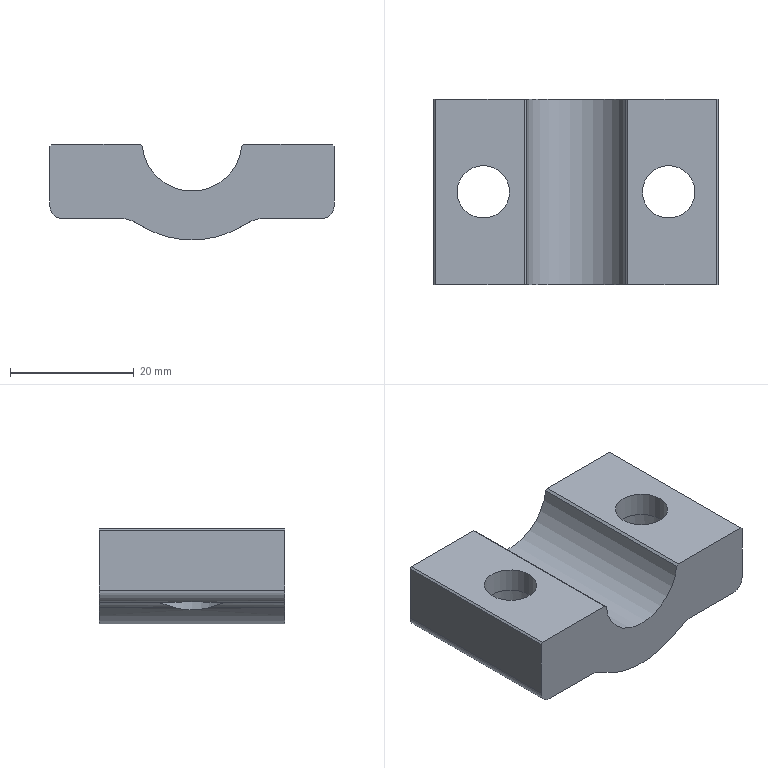NC program | NX | posted with a generic post | part box 46 x 30 x 15.5 mm
Lines 1685 to 1865 of 1865:
(PLANAR_MILL , TOOL : D10精光)
N3362 T03 M6
N3364 G54
N3366 G17 G0 G90 X2.102 Y11.765 B0. C0. S1061 M3
N3368 G43 Z30. H3
N3370 Z-13.5
N3372 G94 G1 Z-15.5 F250.
N3374 G41 X2.208 Y11.595 D3
N3376 G3 X5.033 Y11.456 R2.
N3378 G2 X8.39 Y12.75 R5.
N3380 G1 X22.7
N3382 G2 X26.236 Y11.286 R5.
N3384 G1 X26.536 Y10.986
N3386 G2 X28. Y7.45 R5.
N3388 G1 Y-2.25
N3390 G2 X21. Y-9.25 R7.
N3392 G1 X11.608
N3394 G2 X-11.608 Y-9.25 R21.
N3396 G1 X-21.
N3398 G2 X-28. Y-2.25 R7.
N3400 G1 Y7.45
N3402 G2 X-26.536 Y10.986 R5.
N3404 G1 X-26.236 Y11.286
N3406 G2 X-22.7 Y12.75 R5.
N3408 G1 X-8.39
N3410 G2 X-5.033 Y11.456 R5.
N3412 G1 X-4.704 Y11.157
N3414 G2 X-3.085 Y7.944 R5.
N3416 G3 X3.085 Y7.944 R3.1
N3418 G2 X4.704 Y11.157 R5.
N3420 G1 X5.033 Y11.456
N3422 G3 X5.173 Y14.281 R2.
N3424 G40
N3426 G1 X5.015 Y14.403
N3428 X2.102 Y11.765
N3430 G41 X2.208 Y11.595
N3432 G3 X5.033 Y11.456 R2.
N3434 G2 X8.39 Y12.75 R5.
N3436 G1 X22.7
N3438 G2 X26.236 Y11.286 R5.
N3440 G1 X26.536 Y10.986
N3442 G2 X28. Y7.45 R5.
N3444 G1 Y-2.25
N3446 G2 X21. Y-9.25 R7.
N3448 G1 X11.608
N3450 G2 X-11.608 Y-9.25 R21.
N3452 G1 X-21.
N3454 G2 X-28. Y-2.25 R7.
N3456 G1 Y7.45
N3458 G2 X-26.536 Y10.986 R5.
N3460 G1 X-26.236 Y11.286
N3462 G2 X-22.7 Y12.75 R5.
N3464 G1 X-8.39
N3466 G2 X-5.033 Y11.456 R5.
N3468 G1 X-4.704 Y11.157
N3470 G2 X-3.085 Y7.944 R5.
N3472 G3 X3.085 Y7.944 R3.1
N3474 G2 X4.704 Y11.157 R5.
N3476 G1 X5.033 Y11.456
N3478 G3 X5.173 Y14.281 R2.
N3480 G40
N3482 G1 X5.015 Y14.403
N3484 Z-13.5
N3486 G0 Z30.
N3488 X2.102 Y11.765
N3490 Z-29.
N3492 G1 Z-31.
N3494 G41 X2.208 Y11.595
N3496 G3 X5.033 Y11.456 R2.
N3498 G2 X8.39 Y12.75 R5.
N3500 G1 X22.7
N3502 G2 X26.236 Y11.286 R5.
N3504 G1 X26.536 Y10.986
N3506 G2 X28. Y7.45 R5.
N3508 G1 Y-2.25
N3510 G2 X21. Y-9.25 R7.
N3512 G1 X11.608
N3514 G2 X-11.608 Y-9.25 R21.
N3516 G1 X-21.
N3518 G2 X-28. Y-2.25 R7.
N3520 G1 Y7.45
N3522 G2 X-26.536 Y10.986 R5.
N3524 G1 X-26.236 Y11.286
N3526 G2 X-22.7 Y12.75 R5.
N3528 G1 X-8.39
N3530 G2 X-5.033 Y11.456 R5.
N3532 G1 X-4.704 Y11.157
N3534 G2 X-3.085 Y7.944 R5.
N3536 G3 X3.085 Y7.944 R3.1
N3538 G2 X4.704 Y11.157 R5.
N3540 G1 X5.033 Y11.456
N3542 G3 X5.173 Y14.281 R2.
N3544 G40
N3546 G1 X5.015 Y14.403
N3548 X2.102 Y11.765
N3550 G41 X2.208 Y11.595
N3552 G3 X5.033 Y11.456 R2.
N3554 G2 X8.39 Y12.75 R5.
N3556 G1 X22.7
N3558 G2 X26.236 Y11.286 R5.
N3560 G1 X26.536 Y10.986
N3562 G2 X28. Y7.45 R5.
N3564 G1 Y-2.25
N3566 G2 X21. Y-9.25 R7.
N3568 G1 X11.608
N3570 G2 X-11.608 Y-9.25 R21.
N3572 G1 X-21.
N3574 G2 X-28. Y-2.25 R7.
N3576 G1 Y7.45
N3578 G2 X-26.536 Y10.986 R5.
N3580 G1 X-26.236 Y11.286
N3582 G2 X-22.7 Y12.75 R5.
N3584 G1 X-8.39
N3586 G2 X-5.033 Y11.456 R5.
N3588 G1 X-4.704 Y11.157
N3590 G2 X-3.085 Y7.944 R5.
N3592 G3 X3.085 Y7.944 R3.1
N3594 G2 X4.704 Y11.157 R5.
N3596 G1 X5.033 Y11.456
N3598 G3 X5.173 Y14.281 R2.
N3600 G40
N3602 G1 X5.015 Y14.403
N3604 Z-29.
N3606 G0 Z30.
N3608 M5
(PLANAR_MILL_COPY , TOOL : D10点钻)
N3610 T04 M6
N3612 G54
N3614 G17 G0 G90 X4.222 Y9.372 B0. C0. S3000 M3
N3616 G43 Z30. H4
N3618 Z0.
N3620 G94 G1 Z-2. F800.
N3622 G3 X7.047 Y9.232 R2.
N3624 G2 X8.39 Y9.75 R2.
N3626 G1 X22.7
N3628 G2 X24.114 Y9.164 R2.
N3630 G1 X24.414 Y8.864
N3632 G2 X25. Y7.45 R2.
N3634 G1 Y-2.25
N3636 G2 X21. Y-6.25 R4.
N3638 G1 X11.608
N3640 G3 X9.95 Y-6.75 R3.
N3642 G2 X-9.95 Y-6.75 R18.
N3644 G3 X-11.608 Y-6.25 R3.
N3646 G1 X-21.
N3648 G2 X-25. Y-2.25 R4.
N3650 G1 Y7.45
N3652 G2 X-24.414 Y8.864 R2.
N3654 G1 X-24.114 Y9.164
N3656 G2 X-22.7 Y9.75 R2.
N3658 G1 X-8.39
N3660 G2 X-7.047 Y9.232 R2.
N3662 G1 X-6.718 Y8.934
N3664 G2 X-6.07 Y7.649 R2.
N3666 G3 X6.07 Y7.649 R6.1
N3668 G2 X6.718 Y8.934 R2.
N3670 G1 X7.047 Y9.232
N3672 G3 X7.187 Y12.057 R2.
N3674 G1 Z0.
N3676 G0 Z30.
N3678 M5
(一刀光面_COPY_1 , TOOL : D50R6_1)
N3680 T01 M6
N3682 G54
N3684 G17 G0 G90 X-52.998 Y-1.226 B0. C0. S2000 M3
N3686 G43 Z30. H1
N3688 Z3.
N3690 G94 G1 Z0. F800.
N3692 X-48. Y-1.08
N3694 X48. Y1.739
N3696 X52.998 Y1.886
N3698 Z3.
N3700 G0 Z30.
N3702 M5
N3704 M2